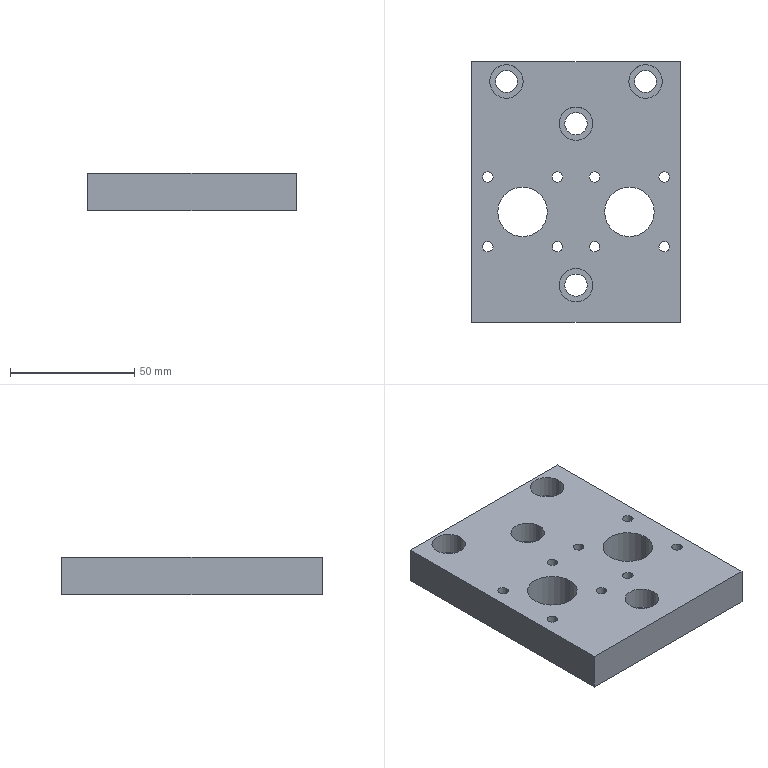Part | STEP file | Printing cylinder fixing plate | 1 solid | 46 faces | box 84 x 105 x 15 mm | volume 114533 mm3 | cylinder 36 | plane 10 | commonest cylinder face diameters 4.2 x16 9 x8 13.5 x8 20 x4
STEP:
#1=CARTESIAN_POINT('',(-9.6,6.,-7.5));
#2=VERTEX_POINT('',#1);
#3=CARTESIAN_POINT('',(-5.4,6.,-7.5));
#4=VERTEX_POINT('',#3);
#5=CARTESIAN_POINT('',(-7.5,6.,-7.5));
#6=DIRECTION('',(0.,0.,1.));
#7=DIRECTION('',(1.,0.,0.));
#8=AXIS2_PLACEMENT_3D('',#5,#6,#7);
#9=CIRCLE('',#8,2.1);
#10=EDGE_CURVE('',#2,#4,#9,.T.);
#11=ORIENTED_EDGE('',*,*,#10,.F.);
#12=CARTESIAN_POINT('',(-9.6,6.,7.5));
#13=VERTEX_POINT('',#12);
#14=CARTESIAN_POINT('',(-9.6,6.,7.5));
#15=DIRECTION('',(0.,0.,1.));
#16=VECTOR('',#15,1000.);
#17=LINE('',#14,#16);
#18=EDGE_CURVE('',#2,#13,#17,.T.);
#19=ORIENTED_EDGE('',*,*,#18,.T.);
#20=CARTESIAN_POINT('',(-5.4,6.,7.5));
#21=VERTEX_POINT('',#20);
#22=CARTESIAN_POINT('',(-7.5,6.,7.5));
#23=DIRECTION('',(0.,0.,1.));
#24=DIRECTION('',(1.,0.,0.));
#25=AXIS2_PLACEMENT_3D('',#22,#23,#24);
#26=CIRCLE('',#25,2.1);
#27=EDGE_CURVE('',#13,#21,#26,.T.);
#28=ORIENTED_EDGE('',*,*,#27,.T.);
#29=CARTESIAN_POINT('',(-5.4,6.,7.5));
#30=DIRECTION('',(0.,0.,1.));
#31=VECTOR('',#30,1000.);
#32=LINE('',#29,#31);
#33=EDGE_CURVE('',#4,#21,#32,.T.);
#34=ORIENTED_EDGE('',*,*,#33,.F.);
#35=EDGE_LOOP('',(#11,#19,#28,#34));
#36=FACE_OUTER_BOUND('',#35,.T.);
#37=CARTESIAN_POINT('',(-7.5,6.,7.5));
#38=DIRECTION('',(0.,0.,1.));
#39=DIRECTION('',(1.,0.,0.));
#40=AXIS2_PLACEMENT_3D('',#37,#38,#39);
#41=CYLINDRICAL_SURFACE('',#40,2.1);
#42=ADVANCED_FACE('',(#36),#41,.F.);
#43=CARTESIAN_POINT('',(-37.6,6.,-7.5));
#44=VERTEX_POINT('',#43);
#45=CARTESIAN_POINT('',(-33.4,6.,-7.5));
#46=VERTEX_POINT('',#45);
#47=CARTESIAN_POINT('',(-35.5,6.,-7.5));
#48=DIRECTION('',(0.,0.,1.));
#49=DIRECTION('',(1.,0.,0.));
#50=AXIS2_PLACEMENT_3D('',#47,#48,#49);
#51=CIRCLE('',#50,2.1);
#52=EDGE_CURVE('',#44,#46,#51,.T.);
#53=ORIENTED_EDGE('',*,*,#52,.F.);
#54=CARTESIAN_POINT('',(-37.6,6.,7.5));
#55=VERTEX_POINT('',#54);
#56=CARTESIAN_POINT('',(-37.6,6.,7.5));
#57=DIRECTION('',(0.,0.,1.));
#58=VECTOR('',#57,1000.);
#59=LINE('',#56,#58);
#60=EDGE_CURVE('',#44,#55,#59,.T.);
#61=ORIENTED_EDGE('',*,*,#60,.T.);
#62=CARTESIAN_POINT('',(-33.4,6.,7.5));
#63=VERTEX_POINT('',#62);
#64=CARTESIAN_POINT('',(-35.5,6.,7.5));
#65=DIRECTION('',(0.,0.,1.));
#66=DIRECTION('',(1.,0.,0.));
#67=AXIS2_PLACEMENT_3D('',#64,#65,#66);
#68=CIRCLE('',#67,2.1);
#69=EDGE_CURVE('',#55,#63,#68,.T.);
#70=ORIENTED_EDGE('',*,*,#69,.T.);
#71=CARTESIAN_POINT('',(-33.4,6.,7.5));
#72=DIRECTION('',(0.,0.,1.));
#73=VECTOR('',#72,1000.);
#74=LINE('',#71,#73);
#75=EDGE_CURVE('',#46,#63,#74,.T.);
#76=ORIENTED_EDGE('',*,*,#75,.F.);
#77=EDGE_LOOP('',(#53,#61,#70,#76));
#78=FACE_OUTER_BOUND('',#77,.T.);
#79=CARTESIAN_POINT('',(-35.5,6.,7.5));
#80=DIRECTION('',(0.,0.,1.));
#81=DIRECTION('',(1.,0.,0.));
#82=AXIS2_PLACEMENT_3D('',#79,#80,#81);
#83=CYLINDRICAL_SURFACE('',#82,2.1);
#84=ADVANCED_FACE('',(#78),#83,.F.);
#85=CARTESIAN_POINT('',(-37.6,-22.,-7.5));
#86=VERTEX_POINT('',#85);
#87=CARTESIAN_POINT('',(-33.4,-22.,-7.5));
#88=VERTEX_POINT('',#87);
#89=CARTESIAN_POINT('',(-35.5,-22.,-7.5));
#90=DIRECTION('',(0.,0.,1.));
#91=DIRECTION('',(1.,0.,0.));
#92=AXIS2_PLACEMENT_3D('',#89,#90,#91);
#93=CIRCLE('',#92,2.1);
#94=EDGE_CURVE('',#86,#88,#93,.T.);
#95=ORIENTED_EDGE('',*,*,#94,.F.);
#96=CARTESIAN_POINT('',(-37.6,-22.,7.5));
#97=VERTEX_POINT('',#96);
#98=CARTESIAN_POINT('',(-37.6,-22.,7.5));
#99=DIRECTION('',(0.,0.,1.));
#100=VECTOR('',#99,1000.);
#101=LINE('',#98,#100);
#102=EDGE_CURVE('',#86,#97,#101,.T.);
#103=ORIENTED_EDGE('',*,*,#102,.T.);
#104=CARTESIAN_POINT('',(-33.4,-22.,7.5));
#105=VERTEX_POINT('',#104);
#106=CARTESIAN_POINT('',(-35.5,-22.,7.5));
#107=DIRECTION('',(0.,0.,1.));
#108=DIRECTION('',(1.,0.,0.));
#109=AXIS2_PLACEMENT_3D('',#106,#107,#108);
#110=CIRCLE('',#109,2.1);
#111=EDGE_CURVE('',#97,#105,#110,.T.);
#112=ORIENTED_EDGE('',*,*,#111,.T.);
#113=CARTESIAN_POINT('',(-33.4,-22.,7.5));
#114=DIRECTION('',(0.,0.,1.));
#115=VECTOR('',#114,1000.);
#116=LINE('',#113,#115);
#117=EDGE_CURVE('',#88,#105,#116,.T.);
#118=ORIENTED_EDGE('',*,*,#117,.F.);
#119=EDGE_LOOP('',(#95,#103,#112,#118));
#120=FACE_OUTER_BOUND('',#119,.T.);
#121=CARTESIAN_POINT('',(-35.5,-22.,7.5));
#122=DIRECTION('',(0.,0.,1.));
#123=DIRECTION('',(1.,0.,0.));
#124=AXIS2_PLACEMENT_3D('',#121,#122,#123);
#125=CYLINDRICAL_SURFACE('',#124,2.1);
#126=ADVANCED_FACE('',(#120),#125,.F.);
#127=CARTESIAN_POINT('',(-9.6,-22.,-7.5));
#128=VERTEX_POINT('',#127);
#129=CARTESIAN_POINT('',(-5.4,-22.,-7.5));
#130=VERTEX_POINT('',#129);
#131=CARTESIAN_POINT('',(-7.5,-22.,-7.5));
#132=DIRECTION('',(0.,0.,1.));
#133=DIRECTION('',(1.,0.,0.));
#134=AXIS2_PLACEMENT_3D('',#131,#132,#133);
#135=CIRCLE('',#134,2.1);
#136=EDGE_CURVE('',#128,#130,#135,.T.);
#137=ORIENTED_EDGE('',*,*,#136,.F.);
#138=CARTESIAN_POINT('',(-9.6,-22.,7.5));
#139=VERTEX_POINT('',#138);
#140=CARTESIAN_POINT('',(-9.6,-22.,7.5));
#141=DIRECTION('',(0.,0.,1.));
#142=VECTOR('',#141,1000.);
#143=LINE('',#140,#142);
#144=EDGE_CURVE('',#128,#139,#143,.T.);
#145=ORIENTED_EDGE('',*,*,#144,.T.);
#146=CARTESIAN_POINT('',(-5.4,-22.,7.5));
#147=VERTEX_POINT('',#146);
#148=CARTESIAN_POINT('',(-7.5,-22.,7.5));
#149=DIRECTION('',(0.,0.,1.));
#150=DIRECTION('',(1.,0.,0.));
#151=AXIS2_PLACEMENT_3D('',#148,#149,#150);
#152=CIRCLE('',#151,2.1);
#153=EDGE_CURVE('',#139,#147,#152,.T.);
#154=ORIENTED_EDGE('',*,*,#153,.T.);
#155=CARTESIAN_POINT('',(-5.4,-22.,7.5));
#156=DIRECTION('',(0.,0.,1.));
#157=VECTOR('',#156,1000.);
#158=LINE('',#155,#157);
#159=EDGE_CURVE('',#130,#147,#158,.T.);
#160=ORIENTED_EDGE('',*,*,#159,.F.);
#161=EDGE_LOOP('',(#137,#145,#154,#160));
#162=FACE_OUTER_BOUND('',#161,.T.);
#163=CARTESIAN_POINT('',(-7.5,-22.,7.5));
#164=DIRECTION('',(0.,0.,1.));
#165=DIRECTION('',(1.,0.,0.));
#166=AXIS2_PLACEMENT_3D('',#163,#164,#165);
#167=CYLINDRICAL_SURFACE('',#166,2.1);
#168=ADVANCED_FACE('',(#162),#167,.F.);
#169=CARTESIAN_POINT('',(5.4,-22.,-7.5));
#170=VERTEX_POINT('',#169);
#171=CARTESIAN_POINT('',(9.6,-22.,-7.5));
#172=VERTEX_POINT('',#171);
#173=CARTESIAN_POINT('',(7.5,-22.,-7.5));
#174=DIRECTION('',(0.,0.,1.));
#175=DIRECTION('',(1.,0.,0.));
#176=AXIS2_PLACEMENT_3D('',#173,#174,#175);
#177=CIRCLE('',#176,2.1);
#178=EDGE_CURVE('',#170,#172,#177,.T.);
#179=ORIENTED_EDGE('',*,*,#178,.F.);
#180=CARTESIAN_POINT('',(5.4,-22.,7.5));
#181=VERTEX_POINT('',#180);
#182=CARTESIAN_POINT('',(5.4,-22.,7.5));
#183=DIRECTION('',(0.,0.,1.));
#184=VECTOR('',#183,1000.);
#185=LINE('',#182,#184);
#186=EDGE_CURVE('',#170,#181,#185,.T.);
#187=ORIENTED_EDGE('',*,*,#186,.T.);
#188=CARTESIAN_POINT('',(9.6,-22.,7.5));
#189=VERTEX_POINT('',#188);
#190=CARTESIAN_POINT('',(7.5,-22.,7.5));
#191=DIRECTION('',(0.,0.,1.));
#192=DIRECTION('',(1.,0.,0.));
#193=AXIS2_PLACEMENT_3D('',#190,#191,#192);
#194=CIRCLE('',#193,2.1);
#195=EDGE_CURVE('',#181,#189,#194,.T.);
#196=ORIENTED_EDGE('',*,*,#195,.T.);
#197=CARTESIAN_POINT('',(9.6,-22.,7.5));
#198=DIRECTION('',(0.,0.,1.));
#199=VECTOR('',#198,1000.);
#200=LINE('',#197,#199);
#201=EDGE_CURVE('',#172,#189,#200,.T.);
#202=ORIENTED_EDGE('',*,*,#201,.F.);
#203=EDGE_LOOP('',(#179,#187,#196,#202));
#204=FACE_OUTER_BOUND('',#203,.T.);
#205=CARTESIAN_POINT('',(7.5,-22.,7.5));
#206=DIRECTION('',(0.,0.,1.));
#207=DIRECTION('',(1.,0.,0.));
#208=AXIS2_PLACEMENT_3D('',#205,#206,#207);
#209=CYLINDRICAL_SURFACE('',#208,2.1);
#210=ADVANCED_FACE('',(#204),#209,.F.);
#211=CARTESIAN_POINT('',(33.4,-22.,-7.5));
#212=VERTEX_POINT('',#211);
#213=CARTESIAN_POINT('',(37.6,-22.,-7.5));
#214=VERTEX_POINT('',#213);
#215=CARTESIAN_POINT('',(35.5,-22.,-7.5));
#216=DIRECTION('',(0.,0.,1.));
#217=DIRECTION('',(1.,0.,0.));
#218=AXIS2_PLACEMENT_3D('',#215,#216,#217);
#219=CIRCLE('',#218,2.1);
#220=EDGE_CURVE('',#212,#214,#219,.T.);
#221=ORIENTED_EDGE('',*,*,#220,.F.);
#222=CARTESIAN_POINT('',(33.4,-22.,7.5));
#223=VERTEX_POINT('',#222);
#224=CARTESIAN_POINT('',(33.4,-22.,7.5));
#225=DIRECTION('',(0.,0.,1.));
#226=VECTOR('',#225,1000.);
#227=LINE('',#224,#226);
#228=EDGE_CURVE('',#212,#223,#227,.T.);
#229=ORIENTED_EDGE('',*,*,#228,.T.);
#230=CARTESIAN_POINT('',(37.6,-22.,7.5));
#231=VERTEX_POINT('',#230);
#232=CARTESIAN_POINT('',(35.5,-22.,7.5));
#233=DIRECTION('',(0.,0.,1.));
#234=DIRECTION('',(1.,0.,0.));
#235=AXIS2_PLACEMENT_3D('',#232,#233,#234);
#236=CIRCLE('',#235,2.1);
#237=EDGE_CURVE('',#223,#231,#236,.T.);
#238=ORIENTED_EDGE('',*,*,#237,.T.);
#239=CARTESIAN_POINT('',(37.6,-22.,7.5));
#240=DIRECTION('',(0.,0.,1.));
#241=VECTOR('',#240,1000.);
#242=LINE('',#239,#241);
#243=EDGE_CURVE('',#214,#231,#242,.T.);
#244=ORIENTED_EDGE('',*,*,#243,.F.);
#245=EDGE_LOOP('',(#221,#229,#238,#244));
#246=FACE_OUTER_BOUND('',#245,.T.);
#247=CARTESIAN_POINT('',(35.5,-22.,7.5));
#248=DIRECTION('',(0.,0.,1.));
#249=DIRECTION('',(1.,0.,0.));
#250=AXIS2_PLACEMENT_3D('',#247,#248,#249);
#251=CYLINDRICAL_SURFACE('',#250,2.1);
#252=ADVANCED_FACE('',(#246),#251,.F.);
#253=CARTESIAN_POINT('',(33.4,6.,-7.5));
#254=VERTEX_POINT('',#253);
#255=CARTESIAN_POINT('',(37.6,6.,-7.5));
#256=VERTEX_POINT('',#255);
#257=CARTESIAN_POINT('',(35.5,6.,-7.5));
#258=DIRECTION('',(0.,0.,1.));
#259=DIRECTION('',(1.,0.,0.));
#260=AXIS2_PLACEMENT_3D('',#257,#258,#259);
#261=CIRCLE('',#260,2.1);
#262=EDGE_CURVE('',#254,#256,#261,.T.);
#263=ORIENTED_EDGE('',*,*,#262,.F.);
#264=CARTESIAN_POINT('',(33.4,6.,7.5));
#265=VERTEX_POINT('',#264);
#266=CARTESIAN_POINT('',(33.4,6.,7.5));
#267=DIRECTION('',(0.,0.,1.));
#268=VECTOR('',#267,1000.);
#269=LINE('',#266,#268);
#270=EDGE_CURVE('',#254,#265,#269,.T.);
#271=ORIENTED_EDGE('',*,*,#270,.T.);
#272=CARTESIAN_POINT('',(37.6,6.,7.5));
#273=VERTEX_POINT('',#272);
#274=CARTESIAN_POINT('',(35.5,6.,7.5));
#275=DIRECTION('',(0.,0.,1.));
#276=DIRECTION('',(1.,0.,0.));
#277=AXIS2_PLACEMENT_3D('',#274,#275,#276);
#278=CIRCLE('',#277,2.1);
#279=EDGE_CURVE('',#265,#273,#278,.T.);
#280=ORIENTED_EDGE('',*,*,#279,.T.);
#281=CARTESIAN_POINT('',(37.6,6.,7.5));
#282=DIRECTION('',(0.,0.,1.));
#283=VECTOR('',#282,1000.);
#284=LINE('',#281,#283);
#285=EDGE_CURVE('',#256,#273,#284,.T.);
#286=ORIENTED_EDGE('',*,*,#285,.F.);
#287=EDGE_LOOP('',(#263,#271,#280,#286));
#288=FACE_OUTER_BOUND('',#287,.T.);
#289=CARTESIAN_POINT('',(35.5,6.,7.5));
#290=DIRECTION('',(0.,0.,1.));
#291=DIRECTION('',(1.,0.,0.));
#292=AXIS2_PLACEMENT_3D('',#289,#290,#291);
#293=CYLINDRICAL_SURFACE('',#292,2.1);
#294=ADVANCED_FACE('',(#288),#293,.F.);
#295=CARTESIAN_POINT('',(5.4,6.,-7.5));
#296=VERTEX_POINT('',#295);
#297=CARTESIAN_POINT('',(9.6,6.,-7.5));
#298=VERTEX_POINT('',#297);
#299=CARTESIAN_POINT('',(7.5,6.,-7.5));
#300=DIRECTION('',(0.,0.,1.));
#301=DIRECTION('',(1.,0.,0.));
#302=AXIS2_PLACEMENT_3D('',#299,#300,#301);
#303=CIRCLE('',#302,2.1);
#304=EDGE_CURVE('',#296,#298,#303,.T.);
#305=ORIENTED_EDGE('',*,*,#304,.F.);
#306=CARTESIAN_POINT('',(5.4,6.,7.5));
#307=VERTEX_POINT('',#306);
#308=CARTESIAN_POINT('',(5.4,6.,7.5));
#309=DIRECTION('',(0.,0.,1.));
#310=VECTOR('',#309,1000.);
#311=LINE('',#308,#310);
#312=EDGE_CURVE('',#296,#307,#311,.T.);
#313=ORIENTED_EDGE('',*,*,#312,.T.);
#314=CARTESIAN_POINT('',(9.6,6.,7.5));
#315=VERTEX_POINT('',#314);
#316=CARTESIAN_POINT('',(7.5,6.,7.5));
#317=DIRECTION('',(0.,0.,1.));
#318=DIRECTION('',(1.,0.,0.));
#319=AXIS2_PLACEMENT_3D('',#316,#317,#318);
#320=CIRCLE('',#319,2.1);
#321=EDGE_CURVE('',#307,#315,#320,.T.);
#322=ORIENTED_EDGE('',*,*,#321,.T.);
#323=CARTESIAN_POINT('',(9.6,6.,7.5));
#324=DIRECTION('',(0.,0.,1.));
#325=VECTOR('',#324,1000.);
#326=LINE('',#323,#325);
#327=EDGE_CURVE('',#298,#315,#326,.T.);
#328=ORIENTED_EDGE('',*,*,#327,.F.);
#329=EDGE_LOOP('',(#305,#313,#322,#328));
#330=FACE_OUTER_BOUND('',#329,.T.);
#331=CARTESIAN_POINT('',(7.5,6.,7.5));
#332=DIRECTION('',(0.,0.,1.));
#333=DIRECTION('',(1.,0.,0.));
#334=AXIS2_PLACEMENT_3D('',#331,#332,#333);
#335=CYLINDRICAL_SURFACE('',#334,2.1);
#336=ADVANCED_FACE('',(#330),#335,.F.);
#337=CARTESIAN_POINT('',(-34.75,44.5,-1.5));
#338=VERTEX_POINT('',#337);
#339=CARTESIAN_POINT('',(-21.25,44.5,-1.5));
#340=VERTEX_POINT('',#339);
#341=CARTESIAN_POINT('',(-28.,44.5,-1.5));
#342=DIRECTION('',(0.,0.,1.));
#343=DIRECTION('',(1.,0.,0.));
#344=AXIS2_PLACEMENT_3D('',#341,#342,#343);
#345=CIRCLE('',#344,6.75);
#346=EDGE_CURVE('',#338,#340,#345,.T.);
#347=ORIENTED_EDGE('',*,*,#346,.F.);
#348=CARTESIAN_POINT('',(-34.75,44.5,7.5));
#349=VERTEX_POINT('',#348);
#350=CARTESIAN_POINT('',(-34.75,44.5,7.5));
#351=DIRECTION('',(0.,0.,1.));
#352=VECTOR('',#351,1000.);
#353=LINE('',#350,#352);
#354=EDGE_CURVE('',#338,#349,#353,.T.);
#355=ORIENTED_EDGE('',*,*,#354,.T.);
#356=CARTESIAN_POINT('',(-21.25,44.5,7.5));
#357=VERTEX_POINT('',#356);
#358=CARTESIAN_POINT('',(-28.,44.5,7.5));
#359=DIRECTION('',(0.,0.,1.));
#360=DIRECTION('',(1.,0.,0.));
#361=AXIS2_PLACEMENT_3D('',#358,#359,#360);
#362=CIRCLE('',#361,6.75);
#363=EDGE_CURVE('',#349,#357,#362,.T.);
#364=ORIENTED_EDGE('',*,*,#363,.T.);
#365=CARTESIAN_POINT('',(-21.25,44.5,7.5));
#366=DIRECTION('',(0.,0.,1.));
#367=VECTOR('',#366,1000.);
#368=LINE('',#365,#367);
#369=EDGE_CURVE('',#340,#357,#368,.T.);
#370=ORIENTED_EDGE('',*,*,#369,.F.);
#371=EDGE_LOOP('',(#347,#355,#364,#370));
#372=FACE_OUTER_BOUND('',#371,.T.);
#373=CARTESIAN_POINT('',(-28.,44.5,7.5));
#374=DIRECTION('',(0.,0.,1.));
#375=DIRECTION('',(1.,0.,0.));
#376=AXIS2_PLACEMENT_3D('',#373,#374,#375);
#377=CYLINDRICAL_SURFACE('',#376,6.75);
#378=ADVANCED_FACE('',(#372),#377,.F.);
#379=CARTESIAN_POINT('',(-32.5,44.5,-7.5));
#380=VERTEX_POINT('',#379);
#381=CARTESIAN_POINT('',(-23.5,44.5,-7.5));
#382=VERTEX_POINT('',#381);
#383=CARTESIAN_POINT('',(-28.,44.5,-7.5));
#384=DIRECTION('',(0.,0.,1.));
#385=DIRECTION('',(1.,0.,0.));
#386=AXIS2_PLACEMENT_3D('',#383,#384,#385);
#387=CIRCLE('',#386,4.5);
#388=EDGE_CURVE('',#380,#382,#387,.T.);
#389=ORIENTED_EDGE('',*,*,#388,.F.);
#390=CARTESIAN_POINT('',(-32.5,44.5,-1.5));
#391=VERTEX_POINT('',#390);
#392=CARTESIAN_POINT('',(-32.5,44.5,7.5));
#393=DIRECTION('',(0.,0.,1.));
#394=VECTOR('',#393,1000.);
#395=LINE('',#392,#394);
#396=EDGE_CURVE('',#380,#391,#395,.T.);
#397=ORIENTED_EDGE('',*,*,#396,.T.);
#398=CARTESIAN_POINT('',(-23.5,44.5,-1.5));
#399=VERTEX_POINT('',#398);
#400=CARTESIAN_POINT('',(-28.,44.5,-1.5));
#401=DIRECTION('',(0.,0.,1.));
#402=DIRECTION('',(1.,0.,0.));
#403=AXIS2_PLACEMENT_3D('',#400,#401,#402);
#404=CIRCLE('',#403,4.5);
#405=EDGE_CURVE('',#391,#399,#404,.T.);
#406=ORIENTED_EDGE('',*,*,#405,.T.);
#407=CARTESIAN_POINT('',(-23.5,44.5,7.5));
#408=DIRECTION('',(0.,0.,1.));
#409=VECTOR('',#408,1000.);
#410=LINE('',#407,#409);
#411=EDGE_CURVE('',#382,#399,#410,.T.);
#412=ORIENTED_EDGE('',*,*,#411,.F.);
#413=EDGE_LOOP('',(#389,#397,#406,#412));
#414=FACE_OUTER_BOUND('',#413,.T.);
#415=CARTESIAN_POINT('',(-28.,44.5,7.5));
#416=DIRECTION('',(0.,0.,1.));
#417=DIRECTION('',(1.,0.,0.));
#418=AXIS2_PLACEMENT_3D('',#415,#416,#417);
#419=CYLINDRICAL_SURFACE('',#418,4.5);
#420=ADVANCED_FACE('',(#414),#419,.F.);
#421=CARTESIAN_POINT('',(21.25,44.5,-1.5));
#422=VERTEX_POINT('',#421);
#423=CARTESIAN_POINT('',(34.75,44.5,-1.5));
#424=VERTEX_POINT('',#423);
#425=CARTESIAN_POINT('',(28.,44.5,-1.5));
#426=DIRECTION('',(0.,0.,1.));
#427=DIRECTION('',(1.,0.,0.));
#428=AXIS2_PLACEMENT_3D('',#425,#426,#427);
#429=CIRCLE('',#428,6.75);
#430=EDGE_CURVE('',#422,#424,#429,.T.);
#431=ORIENTED_EDGE('',*,*,#430,.F.);
#432=CARTESIAN_POINT('',(21.25,44.5,7.5));
#433=VERTEX_POINT('',#432);
#434=CARTESIAN_POINT('',(21.25,44.5,7.5));
#435=DIRECTION('',(0.,0.,1.));
#436=VECTOR('',#435,1000.);
#437=LINE('',#434,#436);
#438=EDGE_CURVE('',#422,#433,#437,.T.);
#439=ORIENTED_EDGE('',*,*,#438,.T.);
#440=CARTESIAN_POINT('',(34.75,44.5,7.5));
#441=VERTEX_POINT('',#440);
#442=CARTESIAN_POINT('',(28.,44.5,7.5));
#443=DIRECTION('',(0.,0.,1.));
#444=DIRECTION('',(1.,0.,0.));
#445=AXIS2_PLACEMENT_3D('',#442,#443,#444);
#446=CIRCLE('',#445,6.75);
#447=EDGE_CURVE('',#433,#441,#446,.T.);
#448=ORIENTED_EDGE('',*,*,#447,.T.);
#449=CARTESIAN_POINT('',(34.75,44.5,7.5));
#450=DIRECTION('',(0.,0.,1.));
#451=VECTOR('',#450,1000.);
#452=LINE('',#449,#451);
#453=EDGE_CURVE('',#424,#441,#452,.T.);
#454=ORIENTED_EDGE('',*,*,#453,.F.);
#455=EDGE_LOOP('',(#431,#439,#448,#454));
#456=FACE_OUTER_BOUND('',#455,.T.);
#457=CARTESIAN_POINT('',(28.,44.5,7.5));
#458=DIRECTION('',(0.,0.,1.));
#459=DIRECTION('',(1.,0.,0.));
#460=AXIS2_PLACEMENT_3D('',#457,#458,#459);
#461=CYLINDRICAL_SURFACE('',#460,6.75);
#462=ADVANCED_FACE('',(#456),#461,.F.);
#463=CARTESIAN_POINT('',(23.5,44.5,-7.5));
#464=VERTEX_POINT('',#463);
#465=CARTESIAN_POINT('',(32.5,44.5,-7.5));
#466=VERTEX_POINT('',#465);
#467=CARTESIAN_POINT('',(28.,44.5,-7.5));
#468=DIRECTION('',(0.,0.,1.));
#469=DIRECTION('',(1.,0.,0.));
#470=AXIS2_PLACEMENT_3D('',#467,#468,#469);
#471=CIRCLE('',#470,4.5);
#472=EDGE_CURVE('',#464,#466,#471,.T.);
#473=ORIENTED_EDGE('',*,*,#472,.F.);
#474=CARTESIAN_POINT('',(23.5,44.5,-1.5));
#475=VERTEX_POINT('',#474);
#476=CARTESIAN_POINT('',(23.5,44.5,7.5));
#477=DIRECTION('',(0.,0.,1.));
#478=VECTOR('',#477,1000.);
#479=LINE('',#476,#478);
#480=EDGE_CURVE('',#464,#475,#479,.T.);
#481=ORIENTED_EDGE('',*,*,#480,.T.);
#482=CARTESIAN_POINT('',(32.5,44.5,-1.5));
#483=VERTEX_POINT('',#482);
#484=CARTESIAN_POINT('',(28.,44.5,-1.5));
#485=DIRECTION('',(0.,0.,1.));
#486=DIRECTION('',(1.,0.,0.));
#487=AXIS2_PLACEMENT_3D('',#484,#485,#486);
#488=CIRCLE('',#487,4.5);
#489=EDGE_CURVE('',#475,#483,#488,.T.);
#490=ORIENTED_EDGE('',*,*,#489,.T.);
#491=CARTESIAN_POINT('',(32.5,44.5,7.5));
#492=DIRECTION('',(0.,0.,1.));
#493=VECTOR('',#492,1000.);
#494=LINE('',#491,#493);
#495=EDGE_CURVE('',#466,#483,#494,.T.);
#496=ORIENTED_EDGE('',*,*,#495,.F.);
#497=EDGE_LOOP('',(#473,#481,#490,#496));
#498=FACE_OUTER_BOUND('',#497,.T.);
#499=CARTESIAN_POINT('',(28.,44.5,7.5));
#500=DIRECTION('',(0.,0.,1.));
#501=DIRECTION('',(1.,0.,0.));
#502=AXIS2_PLACEMENT_3D('',#499,#500,#501);
#503=CYLINDRICAL_SURFACE('',#502,4.5);
#504=ADVANCED_FACE('',(#498),#503,.F.);
#505=CARTESIAN_POINT('',(-6.75,27.5,-1.5));
#506=VERTEX_POINT('',#505);
#507=CARTESIAN_POINT('',(6.75,27.5,-1.5));
#508=VERTEX_POINT('',#507);
#509=CARTESIAN_POINT('',(0.,27.5,-1.5));
#510=DIRECTION('',(0.,0.,1.));
#511=DIRECTION('',(1.,0.,0.));
#512=AXIS2_PLACEMENT_3D('',#509,#510,#511);
#513=CIRCLE('',#512,6.75);
#514=EDGE_CURVE('',#506,#508,#513,.T.);
#515=ORIENTED_EDGE('',*,*,#514,.F.);
#516=CARTESIAN_POINT('',(-6.75,27.5,7.5));
#517=VERTEX_POINT('',#516);
#518=CARTESIAN_POINT('',(-6.75,27.5,7.5));
#519=DIRECTION('',(0.,0.,1.));
#520=VECTOR('',#519,1000.);
#521=LINE('',#518,#520);
#522=EDGE_CURVE('',#506,#517,#521,.T.);
#523=ORIENTED_EDGE('',*,*,#522,.T.);
#524=CARTESIAN_POINT('',(6.75,27.5,7.5));
#525=VERTEX_POINT('',#524);
#526=CARTESIAN_POINT('',(0.,27.5,7.5));
#527=DIRECTION('',(0.,0.,1.));
#528=DIRECTION('',(1.,0.,0.));
#529=AXIS2_PLACEMENT_3D('',#526,#527,#528);
#530=CIRCLE('',#529,6.75);
#531=EDGE_CURVE('',#517,#525,#530,.T.);
#532=ORIENTED_EDGE('',*,*,#531,.T.);
#533=CARTESIAN_POINT('',(6.75,27.5,7.5));
#534=DIRECTION('',(0.,0.,1.));
#535=VECTOR('',#534,1000.);
#536=LINE('',#533,#535);
#537=EDGE_CURVE('',#508,#525,#536,.T.);
#538=ORIENTED_EDGE('',*,*,#537,.F.);
#539=EDGE_LOOP('',(#515,#523,#532,#538));
#540=FACE_OUTER_BOUND('',#539,.T.);
#541=CARTESIAN_POINT('',(0.,27.5,7.5));
#542=DIRECTION('',(0.,0.,1.));
#543=DIRECTION('',(1.,0.,0.));
#544=AXIS2_PLACEMENT_3D('',#541,#542,#543);
#545=CYLINDRICAL_SURFACE('',#544,6.75);
#546=ADVANCED_FACE('',(#540),#545,.F.);
#547=CARTESIAN_POINT('',(-4.5,27.5,-7.5));
#548=VERTEX_POINT('',#547);
#549=CARTESIAN_POINT('',(4.5,27.5,-7.5));
#550=VERTEX_POINT('',#549);
#551=CARTESIAN_POINT('',(0.,27.5,-7.5));
#552=DIRECTION('',(0.,0.,1.));
#553=DIRECTION('',(1.,0.,0.));
#554=AXIS2_PLACEMENT_3D('',#551,#552,#553);
#555=CIRCLE('',#554,4.5);
#556=EDGE_CURVE('',#548,#550,#555,.T.);
#557=ORIENTED_EDGE('',*,*,#556,.F.);
#558=CARTESIAN_POINT('',(-4.5,27.5,-1.5));
#559=VERTEX_POINT('',#558);
#560=CARTESIAN_POINT('',(-4.5,27.5,7.5));
#561=DIRECTION('',(0.,0.,1.));
#562=VECTOR('',#561,1000.);
#563=LINE('',#560,#562);
#564=EDGE_CURVE('',#548,#559,#563,.T.);
#565=ORIENTED_EDGE('',*,*,#564,.T.);
#566=CARTESIAN_POINT('',(4.5,27.5,-1.5));
#567=VERTEX_POINT('',#566);
#568=CARTESIAN_POINT('',(0.,27.5,-1.5));
#569=DIRECTION('',(0.,0.,1.));
#570=DIRECTION('',(1.,0.,0.));
#571=AXIS2_PLACEMENT_3D('',#568,#569,#570);
#572=CIRCLE('',#571,4.5);
#573=EDGE_CURVE('',#559,#567,#572,.T.);
#574=ORIENTED_EDGE('',*,*,#573,.T.);
#575=CARTESIAN_POINT('',(4.5,27.5,7.5));
#576=DIRECTION('',(0.,0.,1.));
#577=VECTOR('',#576,1000.);
#578=LINE('',#575,#577);
#579=EDGE_CURVE('',#550,#567,#578,.T.);
#580=ORIENTED_EDGE('',*,*,#579,.F.);
#581=EDGE_LOOP('',(#557,#565,#574,#580));
#582=FACE_OUTER_BOUND('',#581,.T.);
#583=CARTESIAN_POINT('',(0.,27.5,7.5));
#584=DIRECTION('',(0.,0.,1.));
#585=DIRECTION('',(1.,0.,0.));
#586=AXIS2_PLACEMENT_3D('',#583,#584,#585);
#587=CYLINDRICAL_SURFACE('',#586,4.5);
#588=ADVANCED_FACE('',(#582),#587,.F.);
#589=CARTESIAN_POINT('',(-6.75,-37.5,-1.5));
#590=VERTEX_POINT('',#589);
#591=CARTESIAN_POINT('',(6.75,-37.5,-1.5));
#592=VERTEX_POINT('',#591);
#593=CARTESIAN_POINT('',(0.,-37.5,-1.5));
#594=DIRECTION('',(0.,0.,1.));
#595=DIRECTION('',(1.,0.,0.));
#596=AXIS2_PLACEMENT_3D('',#593,#594,#595);
#597=CIRCLE('',#596,6.75);
#598=EDGE_CURVE('',#590,#592,#597,.T.);
#599=ORIENTED_EDGE('',*,*,#598,.F.);
#600=CARTESIAN_POINT('',(-6.75,-37.5,7.5));
#601=VERTEX_POINT('',#600);
#602=CARTESIAN_POINT('',(-6.75,-37.5,7.5));
#603=DIRECTION('',(0.,0.,1.));
#604=VECTOR('',#603,1000.);
#605=LINE('',#602,#604);
#606=EDGE_CURVE('',#590,#601,#605,.T.);
#607=ORIENTED_EDGE('',*,*,#606,.T.);
#608=CARTESIAN_POINT('',(6.75,-37.5,7.5));
#609=VERTEX_POINT('',#608);
#610=CARTESIAN_POINT('',(0.,-37.5,7.5));
#611=DIRECTION('',(0.,0.,1.));
#612=DIRECTION('',(1.,0.,0.));
#613=AXIS2_PLACEMENT_3D('',#610,#611,#612);
#614=CIRCLE('',#613,6.75);
#615=EDGE_CURVE('',#601,#609,#614,.T.);
#616=ORIENTED_EDGE('',*,*,#615,.T.);
#617=CARTESIAN_POINT('',(6.75,-37.5,7.5));
#618=DIRECTION('',(0.,0.,1.));
#619=VECTOR('',#618,1000.);
#620=LINE('',#617,#619);
#621=EDGE_CURVE('',#592,#609,#620,.T.);
#622=ORIENTED_EDGE('',*,*,#621,.F.);
#623=EDGE_LOOP('',(#599,#607,#616,#622));
#624=FACE_OUTER_BOUND('',#623,.T.);
#625=CARTESIAN_POINT('',(0.,-37.5,7.5));
#626=DIRECTION('',(0.,0.,1.));
#627=DIRECTION('',(1.,0.,0.));
#628=AXIS2_PLACEMENT_3D('',#625,#626,#627);
#629=CYLINDRICAL_SURFACE('',#628,6.75);
#630=ADVANCED_FACE('',(#624),#629,.F.);
#631=CARTESIAN_POINT('',(-4.5,-37.5,-7.5));
#632=VERTEX_POINT('',#631);
#633=CARTESIAN_POINT('',(4.5,-37.5,-7.5));
#634=VERTEX_POINT('',#633);
#635=CARTESIAN_POINT('',(0.,-37.5,-7.5));
#636=DIRECTION('',(0.,0.,1.));
#637=DIRECTION('',(1.,0.,0.));
#638=AXIS2_PLACEMENT_3D('',#635,#636,#637);
#639=CIRCLE('',#638,4.5);
#640=EDGE_CURVE('',#632,#634,#639,.T.);
#641=ORIENTED_EDGE('',*,*,#640,.F.);
#642=CARTESIAN_POINT('',(-4.5,-37.5,-1.5));
#643=VERTEX_POINT('',#642);
#644=CARTESIAN_POINT('',(-4.5,-37.5,7.5));
#645=DIRECTION('',(0.,0.,1.));
#646=VECTOR('',#645,1000.);
#647=LINE('',#644,#646);
#648=EDGE_CURVE('',#632,#643,#647,.T.);
#649=ORIENTED_EDGE('',*,*,#648,.T.);
#650=CARTESIAN_POINT('',(4.5,-37.5,-1.5));
#651=VERTEX_POINT('',#650);
#652=CARTESIAN_POINT('',(0.,-37.5,-1.5));
#653=DIRECTION('',(0.,0.,1.));
#654=DIRECTION('',(1.,0.,0.));
#655=AXIS2_PLACEMENT_3D('',#652,#653,#654);
#656=CIRCLE('',#655,4.5);
#657=EDGE_CURVE('',#643,#651,#656,.T.);
#658=ORIENTED_EDGE('',*,*,#657,.T.);
#659=CARTESIAN_POINT('',(4.5,-37.5,7.5));
#660=DIRECTION('',(0.,0.,1.));
#661=VECTOR('',#660,1000.);
#662=LINE('',#659,#661);
#663=EDGE_CURVE('',#634,#651,#662,.T.);
#664=ORIENTED_EDGE('',*,*,#663,.F.);
#665=EDGE_LOOP('',(#641,#649,#658,#664));
#666=FACE_OUTER_BOUND('',#665,.T.);
#667=CARTESIAN_POINT('',(0.,-37.5,7.5));
#668=DIRECTION('',(0.,0.,1.));
#669=DIRECTION('',(1.,0.,0.));
#670=AXIS2_PLACEMENT_3D('',#667,#668,#669);
#671=CYLINDRICAL_SURFACE('',#670,4.5);
#672=ADVANCED_FACE('',(#666),#671,.F.);
#673=CARTESIAN_POINT('',(-31.5,-8.,-7.5));
#674=VERTEX_POINT('',#673);
#675=CARTESIAN_POINT('',(-11.5,-8.,-7.5));
#676=VERTEX_POINT('',#675);
#677=CARTESIAN_POINT('',(-21.5,-8.,-7.5));
#678=DIRECTION('',(0.,0.,1.));
#679=DIRECTION('',(1.,0.,0.));
#680=AXIS2_PLACEMENT_3D('',#677,#678,#679);
#681=CIRCLE('',#680,10.);
#682=EDGE_CURVE('',#674,#676,#681,.T.);
#683=ORIENTED_EDGE('',*,*,#682,.F.);
#684=CARTESIAN_POINT('',(-31.5,-8.,7.5));
#685=VERTEX_POINT('',#684);
#686=CARTESIAN_POINT('',(-31.5,-8.,-7.5));
#687=DIRECTION('',(0.,0.,1.));
#688=VECTOR('',#687,1000.);
#689=LINE('',#686,#688);
#690=EDGE_CURVE('',#674,#685,#689,.T.);
#691=ORIENTED_EDGE('',*,*,#690,.T.);
#692=CARTESIAN_POINT('',(-11.5,-8.,7.5));
#693=VERTEX_POINT('',#692);
#694=CARTESIAN_POINT('',(-21.5,-8.,7.5));
#695=DIRECTION('',(0.,0.,1.));
#696=DIRECTION('',(1.,0.,0.));
#697=AXIS2_PLACEMENT_3D('',#694,#695,#696);
#698=CIRCLE('',#697,10.);
#699=EDGE_CURVE('',#685,#693,#698,.T.);
#700=ORIENTED_EDGE('',*,*,#699,.T.);
#701=CARTESIAN_POINT('',(-11.5,-8.,-7.5));
#702=DIRECTION('',(0.,0.,1.));
#703=VECTOR('',#702,1000.);
#704=LINE('',#701,#703);
#705=EDGE_CURVE('',#676,#693,#704,.T.);
#706=ORIENTED_EDGE('',*,*,#705,.F.);
#707=EDGE_LOOP('',(#683,#691,#700,#706));
#708=FACE_OUTER_BOUND('',#707,.T.);
#709=CARTESIAN_POINT('',(-21.5,-8.,-7.5));
#710=DIRECTION('',(0.,0.,1.));
#711=DIRECTION('',(1.,0.,0.));
#712=AXIS2_PLACEMENT_3D('',#709,#710,#711);
#713=CYLINDRICAL_SURFACE('',#712,10.);
#714=ADVANCED_FACE('',(#708),#713,.F.);
#715=CARTESIAN_POINT('',(11.5,-8.,-7.5));
#716=VERTEX_POINT('',#715);
#717=CARTESIAN_POINT('',(31.5,-8.,-7.5));
#718=VERTEX_POINT('',#717);
#719=CARTESIAN_POINT('',(21.5,-8.,-7.5));
#720=DIRECTION('',(0.,0.,1.));
#721=DIRECTION('',(1.,0.,0.));
#722=AXIS2_PLACEMENT_3D('',#719,#720,#721);
#723=CIRCLE('',#722,10.);
#724=EDGE_CURVE('',#716,#718,#723,.T.);
#725=ORIENTED_EDGE('',*,*,#724,.F.);
#726=CARTESIAN_POINT('',(11.5,-8.,7.5));
#727=VERTEX_POINT('',#726);
#728=CARTESIAN_POINT('',(11.5,-8.,-7.5));
#729=DIRECTION('',(0.,0.,1.));
#730=VECTOR('',#729,1000.);
#731=LINE('',#728,#730);
#732=EDGE_CURVE('',#716,#727,#731,.T.);
#733=ORIENTED_EDGE('',*,*,#732,.T.);
#734=CARTESIAN_POINT('',(31.5,-8.,7.5));
#735=VERTEX_POINT('',#734);
#736=CARTESIAN_POINT('',(21.5,-8.,7.5));
#737=DIRECTION('',(0.,0.,1.));
#738=DIRECTION('',(1.,0.,0.));
#739=AXIS2_PLACEMENT_3D('',#736,#737,#738);
#740=CIRCLE('',#739,10.);
#741=EDGE_CURVE('',#727,#735,#740,.T.);
#742=ORIENTED_EDGE('',*,*,#741,.T.);
#743=CARTESIAN_POINT('',(31.5,-8.,-7.5));
#744=DIRECTION('',(0.,0.,1.));
#745=VECTOR('',#744,1000.);
#746=LINE('',#743,#745);
#747=EDGE_CURVE('',#718,#735,#746,.T.);
#748=ORIENTED_EDGE('',*,*,#747,.F.);
#749=EDGE_LOOP('',(#725,#733,#742,#748));
#750=FACE_OUTER_BOUND('',#749,.T.);
#751=CARTESIAN_POINT('',(21.5,-8.,-7.5));
#752=DIRECTION('',(0.,0.,1.));
#753=DIRECTION('',(1.,0.,0.));
#754=AXIS2_PLACEMENT_3D('',#751,#752,#753);
#755=CYLINDRICAL_SURFACE('',#754,10.);
#756=ADVANCED_FACE('',(#750),#755,.F.);
#757=CARTESIAN_POINT('',(42.,-52.5,-7.5));
#758=VERTEX_POINT('',#757);
#759=CARTESIAN_POINT('',(42.,52.5,-7.5));
#760=VERTEX_POINT('',#759);
#761=CARTESIAN_POINT('',(42.,52.5,-7.5));
#762=DIRECTION('',(0.,1.,0.));
#763=VECTOR('',#762,1000.);
#764=LINE('',#761,#763);
#765=EDGE_CURVE('',#758,#760,#764,.T.);
#766=ORIENTED_EDGE('',*,*,#765,.T.);
#767=CARTESIAN_POINT('',(42.,52.5,7.5));
#768=VERTEX_POINT('',#767);
#769=CARTESIAN_POINT('',(42.,52.5,7.5));
#770=DIRECTION('',(0.,0.,-1.));
#771=VECTOR('',#770,1000.);
#772=LINE('',#769,#771);
#773=EDGE_CURVE('',#768,#760,#772,.T.);
#774=ORIENTED_EDGE('',*,*,#773,.F.);
#775=CARTESIAN_POINT('',(42.,-52.5,7.5));
#776=VERTEX_POINT('',#775);
#777=CARTESIAN_POINT('',(42.,52.5,7.5));
#778=DIRECTION('',(0.,1.,0.));
#779=VECTOR('',#778,1000.);
#780=LINE('',#777,#779);
#781=EDGE_CURVE('',#776,#768,#780,.T.);
#782=ORIENTED_EDGE('',*,*,#781,.F.);
#783=CARTESIAN_POINT('',(42.,-52.5,7.5));
#784=DIRECTION('',(0.,0.,-1.));
#785=VECTOR('',#784,1000.);
#786=LINE('',#783,#785);
#787=EDGE_CURVE('',#776,#758,#786,.T.);
#788=ORIENTED_EDGE('',*,*,#787,.T.);
#789=EDGE_LOOP('',(#766,#774,#782,#788));
#790=FACE_OUTER_BOUND('',#789,.T.);
#791=CARTESIAN_POINT('',(42.,52.5,7.5));
#792=DIRECTION('',(-1.,0.,0.));
#793=DIRECTION('',(0.,-1.,0.));
#794=AXIS2_PLACEMENT_3D('',#791,#792,#793);
#795=PLANE('',#794);
#796=ADVANCED_FACE('',(#790),#795,.F.);
#797=CARTESIAN_POINT('',(-42.,52.5,-7.5));
#798=VERTEX_POINT('',#797);
#799=CARTESIAN_POINT('',(-42.,52.5,-7.5));
#800=DIRECTION('',(-1.,0.,0.));
#801=VECTOR('',#800,1000.);
#802=LINE('',#799,#801);
#803=EDGE_CURVE('',#760,#798,#802,.T.);
#804=ORIENTED_EDGE('',*,*,#803,.T.);
#805=CARTESIAN_POINT('',(-42.,52.5,7.5));
#806=VERTEX_POINT('',#805);
#807=CARTESIAN_POINT('',(-42.,52.5,7.5));
#808=DIRECTION('',(0.,0.,-1.));
#809=VECTOR('',#808,1000.);
#810=LINE('',#807,#809);
#811=EDGE_CURVE('',#806,#798,#810,.T.);
#812=ORIENTED_EDGE('',*,*,#811,.F.);
#813=CARTESIAN_POINT('',(-42.,52.5,7.5));
#814=DIRECTION('',(-1.,0.,0.));
#815=VECTOR('',#814,1000.);
#816=LINE('',#813,#815);
#817=EDGE_CURVE('',#768,#806,#816,.T.);
#818=ORIENTED_EDGE('',*,*,#817,.F.);
#819=ORIENTED_EDGE('',*,*,#773,.T.);
#820=EDGE_LOOP('',(#804,#812,#818,#819));
#821=FACE_OUTER_BOUND('',#820,.T.);
#822=CARTESIAN_POINT('',(-42.,52.5,7.5));
#823=DIRECTION('',(0.,-1.,0.));
#824=DIRECTION('',(0.,0.,-1.));
#825=AXIS2_PLACEMENT_3D('',#822,#823,#824);
#826=PLANE('',#825);
#827=ADVANCED_FACE('',(#821),#826,.F.);
#828=CARTESIAN_POINT('',(-42.,-52.5,-7.5));
#829=VERTEX_POINT('',#828);
#830=CARTESIAN_POINT('',(-42.,52.5,-7.5));
#831=DIRECTION('',(0.,-1.,0.));
#832=VECTOR('',#831,1000.);
#833=LINE('',#830,#832);
#834=EDGE_CURVE('',#798,#829,#833,.T.);
#835=ORIENTED_EDGE('',*,*,#834,.T.);
#836=CARTESIAN_POINT('',(-42.,-52.5,7.5));
#837=VERTEX_POINT('',#836);
#838=CARTESIAN_POINT('',(-42.,-52.5,7.5));
#839=DIRECTION('',(0.,0.,-1.));
#840=VECTOR('',#839,1000.);
#841=LINE('',#838,#840);
#842=EDGE_CURVE('',#837,#829,#841,.T.);
#843=ORIENTED_EDGE('',*,*,#842,.F.);
#844=CARTESIAN_POINT('',(-42.,52.5,7.5));
#845=DIRECTION('',(0.,-1.,0.));
#846=VECTOR('',#845,1000.);
#847=LINE('',#844,#846);
#848=EDGE_CURVE('',#806,#837,#847,.T.);
#849=ORIENTED_EDGE('',*,*,#848,.F.);
#850=ORIENTED_EDGE('',*,*,#811,.T.);
#851=EDGE_LOOP('',(#835,#843,#849,#850));
#852=FACE_OUTER_BOUND('',#851,.T.);
#853=CARTESIAN_POINT('',(-42.,52.5,7.5));
#854=DIRECTION('',(1.,0.,0.));
#855=DIRECTION('',(0.,1.,0.));
#856=AXIS2_PLACEMENT_3D('',#853,#854,#855);
#857=PLANE('',#856);
#858=ADVANCED_FACE('',(#852),#857,.F.);
#859=CARTESIAN_POINT('',(-42.,-52.5,-7.5));
#860=DIRECTION('',(1.,0.,0.));
#861=VECTOR('',#860,1000.);
#862=LINE('',#859,#861);
#863=EDGE_CURVE('',#829,#758,#862,.T.);
#864=ORIENTED_EDGE('',*,*,#863,.T.);
#865=ORIENTED_EDGE('',*,*,#787,.F.);
#866=CARTESIAN_POINT('',(-42.,-52.5,7.5));
#867=DIRECTION('',(1.,0.,0.));
#868=VECTOR('',#867,1000.);
#869=LINE('',#866,#868);
#870=EDGE_CURVE('',#837,#776,#869,.T.);
#871=ORIENTED_EDGE('',*,*,#870,.F.);
#872=ORIENTED_EDGE('',*,*,#842,.T.);
#873=EDGE_LOOP('',(#864,#865,#871,#872));
#874=FACE_OUTER_BOUND('',#873,.T.);
#875=CARTESIAN_POINT('',(-42.,-52.5,7.5));
#876=DIRECTION('',(0.,1.,0.));
#877=DIRECTION('',(0.,0.,1.));
#878=AXIS2_PLACEMENT_3D('',#875,#876,#877);
#879=PLANE('',#878);
#880=ADVANCED_FACE('',(#874),#879,.F.);
#881=CARTESIAN_POINT('',(-7.5,6.,7.5));
#882=DIRECTION('',(0.,0.,1.));
#883=DIRECTION('',(1.,0.,0.));
#884=AXIS2_PLACEMENT_3D('',#881,#882,#883);
#885=CIRCLE('',#884,2.1);
#886=EDGE_CURVE('',#21,#13,#885,.T.);
#887=ORIENTED_EDGE('',*,*,#886,.F.);
#888=ORIENTED_EDGE('',*,*,#27,.F.);
#889=EDGE_LOOP('',(#887,#888));
#890=FACE_BOUND('',#889,.T.);
#891=CARTESIAN_POINT('',(-35.5,6.,7.5));
#892=DIRECTION('',(0.,0.,1.));
#893=DIRECTION('',(1.,0.,0.));
#894=AXIS2_PLACEMENT_3D('',#891,#892,#893);
#895=CIRCLE('',#894,2.1);
#896=EDGE_CURVE('',#63,#55,#895,.T.);
#897=ORIENTED_EDGE('',*,*,#896,.F.);
#898=ORIENTED_EDGE('',*,*,#69,.F.);
#899=EDGE_LOOP('',(#897,#898));
#900=FACE_BOUND('',#899,.T.);
#901=CARTESIAN_POINT('',(-35.5,-22.,7.5));
#902=DIRECTION('',(0.,0.,1.));
#903=DIRECTION('',(1.,0.,0.));
#904=AXIS2_PLACEMENT_3D('',#901,#902,#903);
#905=CIRCLE('',#904,2.1);
#906=EDGE_CURVE('',#105,#97,#905,.T.);
#907=ORIENTED_EDGE('',*,*,#906,.F.);
#908=ORIENTED_EDGE('',*,*,#111,.F.);
#909=EDGE_LOOP('',(#907,#908));
#910=FACE_BOUND('',#909,.T.);
#911=CARTESIAN_POINT('',(-7.5,-22.,7.5));
#912=DIRECTION('',(0.,0.,1.));
#913=DIRECTION('',(1.,0.,0.));
#914=AXIS2_PLACEMENT_3D('',#911,#912,#913);
#915=CIRCLE('',#914,2.1);
#916=EDGE_CURVE('',#147,#139,#915,.T.);
#917=ORIENTED_EDGE('',*,*,#916,.F.);
#918=ORIENTED_EDGE('',*,*,#153,.F.);
#919=EDGE_LOOP('',(#917,#918));
#920=FACE_BOUND('',#919,.T.);
#921=CARTESIAN_POINT('',(7.5,-22.,7.5));
#922=DIRECTION('',(0.,0.,1.));
#923=DIRECTION('',(1.,0.,0.));
#924=AXIS2_PLACEMENT_3D('',#921,#922,#923);
#925=CIRCLE('',#924,2.1);
#926=EDGE_CURVE('',#189,#181,#925,.T.);
#927=ORIENTED_EDGE('',*,*,#926,.F.);
#928=ORIENTED_EDGE('',*,*,#195,.F.);
#929=EDGE_LOOP('',(#927,#928));
#930=FACE_BOUND('',#929,.T.);
#931=CARTESIAN_POINT('',(35.5,-22.,7.5));
#932=DIRECTION('',(0.,0.,1.));
#933=DIRECTION('',(1.,0.,0.));
#934=AXIS2_PLACEMENT_3D('',#931,#932,#933);
#935=CIRCLE('',#934,2.1);
#936=EDGE_CURVE('',#231,#223,#935,.T.);
#937=ORIENTED_EDGE('',*,*,#936,.F.);
#938=ORIENTED_EDGE('',*,*,#237,.F.);
#939=EDGE_LOOP('',(#937,#938));
#940=FACE_BOUND('',#939,.T.);
#941=CARTESIAN_POINT('',(35.5,6.,7.5));
#942=DIRECTION('',(0.,0.,1.));
#943=DIRECTION('',(1.,0.,0.));
#944=AXIS2_PLACEMENT_3D('',#941,#942,#943);
#945=CIRCLE('',#944,2.1);
#946=EDGE_CURVE('',#273,#265,#945,.T.);
#947=ORIENTED_EDGE('',*,*,#946,.F.);
#948=ORIENTED_EDGE('',*,*,#279,.F.);
#949=EDGE_LOOP('',(#947,#948));
#950=FACE_BOUND('',#949,.T.);
#951=CARTESIAN_POINT('',(7.5,6.,7.5));
#952=DIRECTION('',(0.,0.,1.));
#953=DIRECTION('',(1.,0.,0.));
#954=AXIS2_PLACEMENT_3D('',#951,#952,#953);
#955=CIRCLE('',#954,2.1);
#956=EDGE_CURVE('',#315,#307,#955,.T.);
#957=ORIENTED_EDGE('',*,*,#956,.F.);
#958=ORIENTED_EDGE('',*,*,#321,.F.);
#959=EDGE_LOOP('',(#957,#958));
#960=FACE_BOUND('',#959,.T.);
#961=CARTESIAN_POINT('',(-28.,44.5,7.5));
#962=DIRECTION('',(0.,0.,1.));
#963=DIRECTION('',(1.,0.,0.));
#964=AXIS2_PLACEMENT_3D('',#961,#962,#963);
#965=CIRCLE('',#964,6.75);
#966=EDGE_CURVE('',#357,#349,#965,.T.);
#967=ORIENTED_EDGE('',*,*,#966,.F.);
#968=ORIENTED_EDGE('',*,*,#363,.F.);
#969=EDGE_LOOP('',(#967,#968));
#970=FACE_BOUND('',#969,.T.);
#971=CARTESIAN_POINT('',(28.,44.5,7.5));
#972=DIRECTION('',(0.,0.,1.));
#973=DIRECTION('',(1.,0.,0.));
#974=AXIS2_PLACEMENT_3D('',#971,#972,#973);
#975=CIRCLE('',#974,6.75);
#976=EDGE_CURVE('',#441,#433,#975,.T.);
#977=ORIENTED_EDGE('',*,*,#976,.F.);
#978=ORIENTED_EDGE('',*,*,#447,.F.);
#979=EDGE_LOOP('',(#977,#978));
#980=FACE_BOUND('',#979,.T.);
#981=CARTESIAN_POINT('',(0.,27.5,7.5));
#982=DIRECTION('',(0.,0.,1.));
#983=DIRECTION('',(1.,0.,0.));
#984=AXIS2_PLACEMENT_3D('',#981,#982,#983);
#985=CIRCLE('',#984,6.75);
#986=EDGE_CURVE('',#525,#517,#985,.T.);
#987=ORIENTED_EDGE('',*,*,#986,.F.);
#988=ORIENTED_EDGE('',*,*,#531,.F.);
#989=EDGE_LOOP('',(#987,#988));
#990=FACE_BOUND('',#989,.T.);
#991=CARTESIAN_POINT('',(0.,-37.5,7.5));
#992=DIRECTION('',(0.,0.,1.));
#993=DIRECTION('',(1.,0.,0.));
#994=AXIS2_PLACEMENT_3D('',#991,#992,#993);
#995=CIRCLE('',#994,6.75);
#996=EDGE_CURVE('',#609,#601,#995,.T.);
#997=ORIENTED_EDGE('',*,*,#996,.F.);
#998=ORIENTED_EDGE('',*,*,#615,.F.);
#999=EDGE_LOOP('',(#997,#998));
#1000=FACE_BOUND('',#999,.T.);
#1001=CARTESIAN_POINT('',(-21.5,-8.,7.5));
#1002=DIRECTION('',(0.,0.,1.));
#1003=DIRECTION('',(1.,0.,0.));
#1004=AXIS2_PLACEMENT_3D('',#1001,#1002,#1003);
#1005=CIRCLE('',#1004,10.);
#1006=EDGE_CURVE('',#693,#685,#1005,.T.);
#1007=ORIENTED_EDGE('',*,*,#1006,.F.);
#1008=ORIENTED_EDGE('',*,*,#699,.F.);
#1009=EDGE_LOOP('',(#1007,#1008));
#1010=FACE_BOUND('',#1009,.T.);
#1011=CARTESIAN_POINT('',(21.5,-8.,7.5));
#1012=DIRECTION('',(0.,0.,1.));
#1013=DIRECTION('',(1.,0.,0.));
#1014=AXIS2_PLACEMENT_3D('',#1011,#1012,#1013);
#1015=CIRCLE('',#1014,10.);
#1016=EDGE_CURVE('',#735,#727,#1015,.T.);
#1017=ORIENTED_EDGE('',*,*,#1016,.F.);
#1018=ORIENTED_EDGE('',*,*,#741,.F.);
#1019=EDGE_LOOP('',(#1017,#1018));
#1020=FACE_BOUND('',#1019,.T.);
#1021=ORIENTED_EDGE('',*,*,#781,.T.);
#1022=ORIENTED_EDGE('',*,*,#817,.T.);
#1023=ORIENTED_EDGE('',*,*,#848,.T.);
#1024=ORIENTED_EDGE('',*,*,#870,.T.);
#1025=EDGE_LOOP('',(#1021,#1022,#1023,#1024));
#1026=FACE_OUTER_BOUND('',#1025,.T.);
#1027=CARTESIAN_POINT('',(0.,0.,7.5));
#1028=DIRECTION('',(0.,0.,1.));
#1029=DIRECTION('',(1.,0.,0.));
#1030=AXIS2_PLACEMENT_3D('',#1027,#1028,#1029);
#1031=PLANE('',#1030);
#1032=ADVANCED_FACE('',(#890,#900,#910,#920,#930,#940,#950,#960,#970,#980,#990,#1000,#1010,#1020,#1026),#1031,.T.);
#1033=CARTESIAN_POINT('',(-7.5,6.,-7.5));
#1034=DIRECTION('',(0.,0.,1.));
#1035=DIRECTION('',(1.,0.,0.));
#1036=AXIS2_PLACEMENT_3D('',#1033,#1034,#1035);
#1037=CIRCLE('',#1036,2.1);
#1038=EDGE_CURVE('',#4,#2,#1037,.T.);
#1039=ORIENTED_EDGE('',*,*,#1038,.T.);
#1040=ORIENTED_EDGE('',*,*,#10,.T.);
#1041=EDGE_LOOP('',(#1039,#1040));
#1042=FACE_BOUND('',#1041,.T.);
#1043=CARTESIAN_POINT('',(-35.5,6.,-7.5));
#1044=DIRECTION('',(0.,0.,1.));
#1045=DIRECTION('',(1.,0.,0.));
#1046=AXIS2_PLACEMENT_3D('',#1043,#1044,#1045);
#1047=CIRCLE('',#1046,2.1);
#1048=EDGE_CURVE('',#46,#44,#1047,.T.);
#1049=ORIENTED_EDGE('',*,*,#1048,.T.);
#1050=ORIENTED_EDGE('',*,*,#52,.T.);
#1051=EDGE_LOOP('',(#1049,#1050));
#1052=FACE_BOUND('',#1051,.T.);
#1053=CARTESIAN_POINT('',(-35.5,-22.,-7.5));
#1054=DIRECTION('',(0.,0.,1.));
#1055=DIRECTION('',(1.,0.,0.));
#1056=AXIS2_PLACEMENT_3D('',#1053,#1054,#1055);
#1057=CIRCLE('',#1056,2.1);
#1058=EDGE_CURVE('',#88,#86,#1057,.T.);
#1059=ORIENTED_EDGE('',*,*,#1058,.T.);
#1060=ORIENTED_EDGE('',*,*,#94,.T.);
#1061=EDGE_LOOP('',(#1059,#1060));
#1062=FACE_BOUND('',#1061,.T.);
#1063=CARTESIAN_POINT('',(-7.5,-22.,-7.5));
#1064=DIRECTION('',(0.,0.,1.));
#1065=DIRECTION('',(1.,0.,0.));
#1066=AXIS2_PLACEMENT_3D('',#1063,#1064,#1065);
#1067=CIRCLE('',#1066,2.1);
#1068=EDGE_CURVE('',#130,#128,#1067,.T.);
#1069=ORIENTED_EDGE('',*,*,#1068,.T.);
#1070=ORIENTED_EDGE('',*,*,#136,.T.);
#1071=EDGE_LOOP('',(#1069,#1070));
#1072=FACE_BOUND('',#1071,.T.);
#1073=CARTESIAN_POINT('',(7.5,-22.,-7.5));
#1074=DIRECTION('',(0.,0.,1.));
#1075=DIRECTION('',(1.,0.,0.));
#1076=AXIS2_PLACEMENT_3D('',#1073,#1074,#1075);
#1077=CIRCLE('',#1076,2.1);
#1078=EDGE_CURVE('',#172,#170,#1077,.T.);
#1079=ORIENTED_EDGE('',*,*,#1078,.T.);
#1080=ORIENTED_EDGE('',*,*,#178,.T.);
#1081=EDGE_LOOP('',(#1079,#1080));
#1082=FACE_BOUND('',#1081,.T.);
#1083=CARTESIAN_POINT('',(35.5,-22.,-7.5));
#1084=DIRECTION('',(0.,0.,1.));
#1085=DIRECTION('',(1.,0.,0.));
#1086=AXIS2_PLACEMENT_3D('',#1083,#1084,#1085);
#1087=CIRCLE('',#1086,2.1);
#1088=EDGE_CURVE('',#214,#212,#1087,.T.);
#1089=ORIENTED_EDGE('',*,*,#1088,.T.);
#1090=ORIENTED_EDGE('',*,*,#220,.T.);
#1091=EDGE_LOOP('',(#1089,#1090));
#1092=FACE_BOUND('',#1091,.T.);
#1093=CARTESIAN_POINT('',(35.5,6.,-7.5));
#1094=DIRECTION('',(0.,0.,1.));
#1095=DIRECTION('',(1.,0.,0.));
#1096=AXIS2_PLACEMENT_3D('',#1093,#1094,#1095);
#1097=CIRCLE('',#1096,2.1);
#1098=EDGE_CURVE('',#256,#254,#1097,.T.);
#1099=ORIENTED_EDGE('',*,*,#1098,.T.);
#1100=ORIENTED_EDGE('',*,*,#262,.T.);
#1101=EDGE_LOOP('',(#1099,#1100));
#1102=FACE_BOUND('',#1101,.T.);
#1103=CARTESIAN_POINT('',(7.5,6.,-7.5));
#1104=DIRECTION('',(0.,0.,1.));
#1105=DIRECTION('',(1.,0.,0.));
#1106=AXIS2_PLACEMENT_3D('',#1103,#1104,#1105);
#1107=CIRCLE('',#1106,2.1);
#1108=EDGE_CURVE('',#298,#296,#1107,.T.);
#1109=ORIENTED_EDGE('',*,*,#1108,.T.);
#1110=ORIENTED_EDGE('',*,*,#304,.T.);
#1111=EDGE_LOOP('',(#1109,#1110));
#1112=FACE_BOUND('',#1111,.T.);
#1113=CARTESIAN_POINT('',(-28.,44.5,-7.5));
#1114=DIRECTION('',(0.,0.,1.));
#1115=DIRECTION('',(1.,0.,0.));
#1116=AXIS2_PLACEMENT_3D('',#1113,#1114,#1115);
#1117=CIRCLE('',#1116,4.5);
#1118=EDGE_CURVE('',#382,#380,#1117,.T.);
#1119=ORIENTED_EDGE('',*,*,#1118,.T.);
#1120=ORIENTED_EDGE('',*,*,#388,.T.);
#1121=EDGE_LOOP('',(#1119,#1120));
#1122=FACE_BOUND('',#1121,.T.);
#1123=CARTESIAN_POINT('',(28.,44.5,-7.5));
#1124=DIRECTION('',(0.,0.,1.));
#1125=DIRECTION('',(1.,0.,0.));
#1126=AXIS2_PLACEMENT_3D('',#1123,#1124,#1125);
#1127=CIRCLE('',#1126,4.5);
#1128=EDGE_CURVE('',#466,#464,#1127,.T.);
#1129=ORIENTED_EDGE('',*,*,#1128,.T.);
#1130=ORIENTED_EDGE('',*,*,#472,.T.);
#1131=EDGE_LOOP('',(#1129,#1130));
#1132=FACE_BOUND('',#1131,.T.);
#1133=CARTESIAN_POINT('',(0.,27.5,-7.5));
#1134=DIRECTION('',(0.,0.,1.));
#1135=DIRECTION('',(1.,0.,0.));
#1136=AXIS2_PLACEMENT_3D('',#1133,#1134,#1135);
#1137=CIRCLE('',#1136,4.5);
#1138=EDGE_CURVE('',#550,#548,#1137,.T.);
#1139=ORIENTED_EDGE('',*,*,#1138,.T.);
#1140=ORIENTED_EDGE('',*,*,#556,.T.);
#1141=EDGE_LOOP('',(#1139,#1140));
#1142=FACE_BOUND('',#1141,.T.);
#1143=CARTESIAN_POINT('',(0.,-37.5,-7.5));
#1144=DIRECTION('',(0.,0.,1.));
#1145=DIRECTION('',(1.,0.,0.));
#1146=AXIS2_PLACEMENT_3D('',#1143,#1144,#1145);
#1147=CIRCLE('',#1146,4.5);
#1148=EDGE_CURVE('',#634,#632,#1147,.T.);
#1149=ORIENTED_EDGE('',*,*,#1148,.T.);
#1150=ORIENTED_EDGE('',*,*,#640,.T.);
#1151=EDGE_LOOP('',(#1149,#1150));
#1152=FACE_BOUND('',#1151,.T.);
#1153=CARTESIAN_POINT('',(-21.5,-8.,-7.5));
#1154=DIRECTION('',(0.,0.,1.));
#1155=DIRECTION('',(1.,0.,0.));
#1156=AXIS2_PLACEMENT_3D('',#1153,#1154,#1155);
#1157=CIRCLE('',#1156,10.);
#1158=EDGE_CURVE('',#676,#674,#1157,.T.);
#1159=ORIENTED_EDGE('',*,*,#1158,.T.);
#1160=ORIENTED_EDGE('',*,*,#682,.T.);
#1161=EDGE_LOOP('',(#1159,#1160));
#1162=FACE_BOUND('',#1161,.T.);
#1163=CARTESIAN_POINT('',(21.5,-8.,-7.5));
#1164=DIRECTION('',(0.,0.,1.));
#1165=DIRECTION('',(1.,0.,0.));
#1166=AXIS2_PLACEMENT_3D('',#1163,#1164,#1165);
#1167=CIRCLE('',#1166,10.);
#1168=EDGE_CURVE('',#718,#716,#1167,.T.);
#1169=ORIENTED_EDGE('',*,*,#1168,.T.);
#1170=ORIENTED_EDGE('',*,*,#724,.T.);
#1171=EDGE_LOOP('',(#1169,#1170));
#1172=FACE_BOUND('',#1171,.T.);
#1173=ORIENTED_EDGE('',*,*,#765,.F.);
#1174=ORIENTED_EDGE('',*,*,#863,.F.);
#1175=ORIENTED_EDGE('',*,*,#834,.F.);
#1176=ORIENTED_EDGE('',*,*,#803,.F.);
#1177=EDGE_LOOP('',(#1173,#1174,#1175,#1176));
#1178=FACE_OUTER_BOUND('',#1177,.T.);
#1179=CARTESIAN_POINT('',(0.,0.,-7.5));
#1180=DIRECTION('',(0.,0.,1.));
#1181=DIRECTION('',(1.,0.,0.));
#1182=AXIS2_PLACEMENT_3D('',#1179,#1180,#1181);
#1183=PLANE('',#1182);
#1184=ADVANCED_FACE('',(#1042,#1052,#1062,#1072,#1082,#1092,#1102,#1112,#1122,#1132,#1142,#1152,#1162,#1172,#1178),#1183,.F.);
#1185=ORIENTED_EDGE('',*,*,#732,.F.);
#1186=ORIENTED_EDGE('',*,*,#1168,.F.);
#1187=ORIENTED_EDGE('',*,*,#747,.T.);
#1188=ORIENTED_EDGE('',*,*,#1016,.T.);
#1189=EDGE_LOOP('',(#1185,#1186,#1187,#1188));
#1190=FACE_OUTER_BOUND('',#1189,.T.);
#1191=CARTESIAN_POINT('',(21.5,-8.,-7.5));
#1192=DIRECTION('',(0.,0.,1.));
#1193=DIRECTION('',(1.,0.,0.));
#1194=AXIS2_PLACEMENT_3D('',#1191,#1192,#1193);
#1195=CYLINDRICAL_SURFACE('',#1194,10.);
#1196=ADVANCED_FACE('',(#1190),#1195,.F.);
#1197=ORIENTED_EDGE('',*,*,#690,.F.);
#1198=ORIENTED_EDGE('',*,*,#1158,.F.);
#1199=ORIENTED_EDGE('',*,*,#705,.T.);
#1200=ORIENTED_EDGE('',*,*,#1006,.T.);
#1201=EDGE_LOOP('',(#1197,#1198,#1199,#1200));
#1202=FACE_OUTER_BOUND('',#1201,.T.);
#1203=CARTESIAN_POINT('',(-21.5,-8.,-7.5));
#1204=DIRECTION('',(0.,0.,1.));
#1205=DIRECTION('',(1.,0.,0.));
#1206=AXIS2_PLACEMENT_3D('',#1203,#1204,#1205);
#1207=CYLINDRICAL_SURFACE('',#1206,10.);
#1208=ADVANCED_FACE('',(#1202),#1207,.F.);
#1209=ORIENTED_EDGE('',*,*,#648,.F.);
#1210=ORIENTED_EDGE('',*,*,#1148,.F.);
#1211=ORIENTED_EDGE('',*,*,#663,.T.);
#1212=CARTESIAN_POINT('',(0.,-37.5,-1.5));
#1213=DIRECTION('',(0.,0.,1.));
#1214=DIRECTION('',(1.,0.,0.));
#1215=AXIS2_PLACEMENT_3D('',#1212,#1213,#1214);
#1216=CIRCLE('',#1215,4.5);
#1217=EDGE_CURVE('',#651,#643,#1216,.T.);
#1218=ORIENTED_EDGE('',*,*,#1217,.T.);
#1219=EDGE_LOOP('',(#1209,#1210,#1211,#1218));
#1220=FACE_OUTER_BOUND('',#1219,.T.);
#1221=CARTESIAN_POINT('',(0.,-37.5,7.5));
#1222=DIRECTION('',(0.,0.,1.));
#1223=DIRECTION('',(1.,0.,0.));
#1224=AXIS2_PLACEMENT_3D('',#1221,#1222,#1223);
#1225=CYLINDRICAL_SURFACE('',#1224,4.5);
#1226=ADVANCED_FACE('',(#1220),#1225,.F.);
#1227=ORIENTED_EDGE('',*,*,#1217,.F.);
#1228=ORIENTED_EDGE('',*,*,#657,.F.);
#1229=EDGE_LOOP('',(#1227,#1228));
#1230=FACE_BOUND('',#1229,.T.);
#1231=CARTESIAN_POINT('',(0.,-37.5,-1.5));
#1232=DIRECTION('',(0.,0.,1.));
#1233=DIRECTION('',(1.,0.,0.));
#1234=AXIS2_PLACEMENT_3D('',#1231,#1232,#1233);
#1235=CIRCLE('',#1234,6.75);
#1236=EDGE_CURVE('',#592,#590,#1235,.T.);
#1237=ORIENTED_EDGE('',*,*,#1236,.T.);
#1238=ORIENTED_EDGE('',*,*,#598,.T.);
#1239=EDGE_LOOP('',(#1237,#1238));
#1240=FACE_OUTER_BOUND('',#1239,.T.);
#1241=CARTESIAN_POINT('',(4.5,-37.5,-1.5));
#1242=DIRECTION('',(0.,0.,-1.));
#1243=DIRECTION('',(-1.,0.,0.));
#1244=AXIS2_PLACEMENT_3D('',#1241,#1242,#1243);
#1245=PLANE('',#1244);
#1246=ADVANCED_FACE('',(#1230,#1240),#1245,.F.);
#1247=ORIENTED_EDGE('',*,*,#606,.F.);
#1248=ORIENTED_EDGE('',*,*,#1236,.F.);
#1249=ORIENTED_EDGE('',*,*,#621,.T.);
#1250=ORIENTED_EDGE('',*,*,#996,.T.);
#1251=EDGE_LOOP('',(#1247,#1248,#1249,#1250));
#1252=FACE_OUTER_BOUND('',#1251,.T.);
#1253=CARTESIAN_POINT('',(0.,-37.5,7.5));
#1254=DIRECTION('',(0.,0.,1.));
#1255=DIRECTION('',(1.,0.,0.));
#1256=AXIS2_PLACEMENT_3D('',#1253,#1254,#1255);
#1257=CYLINDRICAL_SURFACE('',#1256,6.75);
#1258=ADVANCED_FACE('',(#1252),#1257,.F.);
#1259=ORIENTED_EDGE('',*,*,#564,.F.);
#1260=ORIENTED_EDGE('',*,*,#1138,.F.);
#1261=ORIENTED_EDGE('',*,*,#579,.T.);
#1262=CARTESIAN_POINT('',(0.,27.5,-1.5));
#1263=DIRECTION('',(0.,0.,1.));
#1264=DIRECTION('',(1.,0.,0.));
#1265=AXIS2_PLACEMENT_3D('',#1262,#1263,#1264);
#1266=CIRCLE('',#1265,4.5);
#1267=EDGE_CURVE('',#567,#559,#1266,.T.);
#1268=ORIENTED_EDGE('',*,*,#1267,.T.);
#1269=EDGE_LOOP('',(#1259,#1260,#1261,#1268));
#1270=FACE_OUTER_BOUND('',#1269,.T.);
#1271=CARTESIAN_POINT('',(0.,27.5,7.5));
#1272=DIRECTION('',(0.,0.,1.));
#1273=DIRECTION('',(1.,0.,0.));
#1274=AXIS2_PLACEMENT_3D('',#1271,#1272,#1273);
#1275=CYLINDRICAL_SURFACE('',#1274,4.5);
#1276=ADVANCED_FACE('',(#1270),#1275,.F.);
#1277=ORIENTED_EDGE('',*,*,#1267,.F.);
#1278=ORIENTED_EDGE('',*,*,#573,.F.);
#1279=EDGE_LOOP('',(#1277,#1278));
#1280=FACE_BOUND('',#1279,.T.);
#1281=CARTESIAN_POINT('',(0.,27.5,-1.5));
#1282=DIRECTION('',(0.,0.,1.));
#1283=DIRECTION('',(1.,0.,0.));
#1284=AXIS2_PLACEMENT_3D('',#1281,#1282,#1283);
#1285=CIRCLE('',#1284,6.75);
#1286=EDGE_CURVE('',#508,#506,#1285,.T.);
#1287=ORIENTED_EDGE('',*,*,#1286,.T.);
#1288=ORIENTED_EDGE('',*,*,#514,.T.);
#1289=EDGE_LOOP('',(#1287,#1288));
#1290=FACE_OUTER_BOUND('',#1289,.T.);
#1291=CARTESIAN_POINT('',(4.5,27.5,-1.5));
#1292=DIRECTION('',(0.,0.,-1.));
#1293=DIRECTION('',(-1.,0.,0.));
#1294=AXIS2_PLACEMENT_3D('',#1291,#1292,#1293);
#1295=PLANE('',#1294);
#1296=ADVANCED_FACE('',(#1280,#1290),#1295,.F.);
#1297=ORIENTED_EDGE('',*,*,#522,.F.);
#1298=ORIENTED_EDGE('',*,*,#1286,.F.);
#1299=ORIENTED_EDGE('',*,*,#537,.T.);
#1300=ORIENTED_EDGE('',*,*,#986,.T.);
#1301=EDGE_LOOP('',(#1297,#1298,#1299,#1300));
#1302=FACE_OUTER_BOUND('',#1301,.T.);
#1303=CARTESIAN_POINT('',(0.,27.5,7.5));
#1304=DIRECTION('',(0.,0.,1.));
#1305=DIRECTION('',(1.,0.,0.));
#1306=AXIS2_PLACEMENT_3D('',#1303,#1304,#1305);
#1307=CYLINDRICAL_SURFACE('',#1306,6.75);
#1308=ADVANCED_FACE('',(#1302),#1307,.F.);
#1309=ORIENTED_EDGE('',*,*,#480,.F.);
#1310=ORIENTED_EDGE('',*,*,#1128,.F.);
#1311=ORIENTED_EDGE('',*,*,#495,.T.);
#1312=CARTESIAN_POINT('',(28.,44.5,-1.5));
#1313=DIRECTION('',(0.,0.,1.));
#1314=DIRECTION('',(1.,0.,0.));
#1315=AXIS2_PLACEMENT_3D('',#1312,#1313,#1314);
#1316=CIRCLE('',#1315,4.5);
#1317=EDGE_CURVE('',#483,#475,#1316,.T.);
#1318=ORIENTED_EDGE('',*,*,#1317,.T.);
#1319=EDGE_LOOP('',(#1309,#1310,#1311,#1318));
#1320=FACE_OUTER_BOUND('',#1319,.T.);
#1321=CARTESIAN_POINT('',(28.,44.5,7.5));
#1322=DIRECTION('',(0.,0.,1.));
#1323=DIRECTION('',(1.,0.,0.));
#1324=AXIS2_PLACEMENT_3D('',#1321,#1322,#1323);
#1325=CYLINDRICAL_SURFACE('',#1324,4.5);
#1326=ADVANCED_FACE('',(#1320),#1325,.F.);
#1327=ORIENTED_EDGE('',*,*,#1317,.F.);
#1328=ORIENTED_EDGE('',*,*,#489,.F.);
#1329=EDGE_LOOP('',(#1327,#1328));
#1330=FACE_BOUND('',#1329,.T.);
#1331=CARTESIAN_POINT('',(28.,44.5,-1.5));
#1332=DIRECTION('',(0.,0.,1.));
#1333=DIRECTION('',(1.,0.,0.));
#1334=AXIS2_PLACEMENT_3D('',#1331,#1332,#1333);
#1335=CIRCLE('',#1334,6.75);
#1336=EDGE_CURVE('',#424,#422,#1335,.T.);
#1337=ORIENTED_EDGE('',*,*,#1336,.T.);
#1338=ORIENTED_EDGE('',*,*,#430,.T.);
#1339=EDGE_LOOP('',(#1337,#1338));
#1340=FACE_OUTER_BOUND('',#1339,.T.);
#1341=CARTESIAN_POINT('',(32.5,44.5,-1.5));
#1342=DIRECTION('',(0.,0.,-1.));
#1343=DIRECTION('',(-1.,0.,0.));
#1344=AXIS2_PLACEMENT_3D('',#1341,#1342,#1343);
#1345=PLANE('',#1344);
#1346=ADVANCED_FACE('',(#1330,#1340),#1345,.F.);
#1347=ORIENTED_EDGE('',*,*,#438,.F.);
#1348=ORIENTED_EDGE('',*,*,#1336,.F.);
#1349=ORIENTED_EDGE('',*,*,#453,.T.);
#1350=ORIENTED_EDGE('',*,*,#976,.T.);
#1351=EDGE_LOOP('',(#1347,#1348,#1349,#1350));
#1352=FACE_OUTER_BOUND('',#1351,.T.);
#1353=CARTESIAN_POINT('',(28.,44.5,7.5));
#1354=DIRECTION('',(0.,0.,1.));
#1355=DIRECTION('',(1.,0.,0.));
#1356=AXIS2_PLACEMENT_3D('',#1353,#1354,#1355);
#1357=CYLINDRICAL_SURFACE('',#1356,6.75);
#1358=ADVANCED_FACE('',(#1352),#1357,.F.);
#1359=ORIENTED_EDGE('',*,*,#396,.F.);
#1360=ORIENTED_EDGE('',*,*,#1118,.F.);
#1361=ORIENTED_EDGE('',*,*,#411,.T.);
#1362=CARTESIAN_POINT('',(-28.,44.5,-1.5));
#1363=DIRECTION('',(0.,0.,1.));
#1364=DIRECTION('',(1.,0.,0.));
#1365=AXIS2_PLACEMENT_3D('',#1362,#1363,#1364);
#1366=CIRCLE('',#1365,4.5);
#1367=EDGE_CURVE('',#399,#391,#1366,.T.);
#1368=ORIENTED_EDGE('',*,*,#1367,.T.);
#1369=EDGE_LOOP('',(#1359,#1360,#1361,#1368));
#1370=FACE_OUTER_BOUND('',#1369,.T.);
#1371=CARTESIAN_POINT('',(-28.,44.5,7.5));
#1372=DIRECTION('',(0.,0.,1.));
#1373=DIRECTION('',(1.,0.,0.));
#1374=AXIS2_PLACEMENT_3D('',#1371,#1372,#1373);
#1375=CYLINDRICAL_SURFACE('',#1374,4.5);
#1376=ADVANCED_FACE('',(#1370),#1375,.F.);
#1377=ORIENTED_EDGE('',*,*,#1367,.F.);
#1378=ORIENTED_EDGE('',*,*,#405,.F.);
#1379=EDGE_LOOP('',(#1377,#1378));
#1380=FACE_BOUND('',#1379,.T.);
#1381=CARTESIAN_POINT('',(-28.,44.5,-1.5));
#1382=DIRECTION('',(0.,0.,1.));
#1383=DIRECTION('',(1.,0.,0.));
#1384=AXIS2_PLACEMENT_3D('',#1381,#1382,#1383);
#1385=CIRCLE('',#1384,6.75);
#1386=EDGE_CURVE('',#340,#338,#1385,.T.);
#1387=ORIENTED_EDGE('',*,*,#1386,.T.);
#1388=ORIENTED_EDGE('',*,*,#346,.T.);
#1389=EDGE_LOOP('',(#1387,#1388));
#1390=FACE_OUTER_BOUND('',#1389,.T.);
#1391=CARTESIAN_POINT('',(-23.5,44.5,-1.5));
#1392=DIRECTION('',(0.,0.,-1.));
#1393=DIRECTION('',(-1.,0.,0.));
#1394=AXIS2_PLACEMENT_3D('',#1391,#1392,#1393);
#1395=PLANE('',#1394);
#1396=ADVANCED_FACE('',(#1380,#1390),#1395,.F.);
#1397=ORIENTED_EDGE('',*,*,#354,.F.);
#1398=ORIENTED_EDGE('',*,*,#1386,.F.);
#1399=ORIENTED_EDGE('',*,*,#369,.T.);
#1400=ORIENTED_EDGE('',*,*,#966,.T.);
#1401=EDGE_LOOP('',(#1397,#1398,#1399,#1400));
#1402=FACE_OUTER_BOUND('',#1401,.T.);
#1403=CARTESIAN_POINT('',(-28.,44.5,7.5));
#1404=DIRECTION('',(0.,0.,1.));
#1405=DIRECTION('',(1.,0.,0.));
#1406=AXIS2_PLACEMENT_3D('',#1403,#1404,#1405);
#1407=CYLINDRICAL_SURFACE('',#1406,6.75);
#1408=ADVANCED_FACE('',(#1402),#1407,.F.);
#1409=ORIENTED_EDGE('',*,*,#312,.F.);
#1410=ORIENTED_EDGE('',*,*,#1108,.F.);
#1411=ORIENTED_EDGE('',*,*,#327,.T.);
#1412=ORIENTED_EDGE('',*,*,#956,.T.);
#1413=EDGE_LOOP('',(#1409,#1410,#1411,#1412));
#1414=FACE_OUTER_BOUND('',#1413,.T.);
#1415=CARTESIAN_POINT('',(7.5,6.,7.5));
#1416=DIRECTION('',(0.,0.,1.));
#1417=DIRECTION('',(1.,0.,0.));
#1418=AXIS2_PLACEMENT_3D('',#1415,#1416,#1417);
#1419=CYLINDRICAL_SURFACE('',#1418,2.1);
#1420=ADVANCED_FACE('',(#1414),#1419,.F.);
#1421=ORIENTED_EDGE('',*,*,#270,.F.);
#1422=ORIENTED_EDGE('',*,*,#1098,.F.);
#1423=ORIENTED_EDGE('',*,*,#285,.T.);
#1424=ORIENTED_EDGE('',*,*,#946,.T.);
#1425=EDGE_LOOP('',(#1421,#1422,#1423,#1424));
#1426=FACE_OUTER_BOUND('',#1425,.T.);
#1427=CARTESIAN_POINT('',(35.5,6.,7.5));
#1428=DIRECTION('',(0.,0.,1.));
#1429=DIRECTION('',(1.,0.,0.));
#1430=AXIS2_PLACEMENT_3D('',#1427,#1428,#1429);
#1431=CYLINDRICAL_SURFACE('',#1430,2.1);
#1432=ADVANCED_FACE('',(#1426),#1431,.F.);
#1433=ORIENTED_EDGE('',*,*,#228,.F.);
#1434=ORIENTED_EDGE('',*,*,#1088,.F.);
#1435=ORIENTED_EDGE('',*,*,#243,.T.);
#1436=ORIENTED_EDGE('',*,*,#936,.T.);
#1437=EDGE_LOOP('',(#1433,#1434,#1435,#1436));
#1438=FACE_OUTER_BOUND('',#1437,.T.);
#1439=CARTESIAN_POINT('',(35.5,-22.,7.5));
#1440=DIRECTION('',(0.,0.,1.));
#1441=DIRECTION('',(1.,0.,0.));
#1442=AXIS2_PLACEMENT_3D('',#1439,#1440,#1441);
#1443=CYLINDRICAL_SURFACE('',#1442,2.1);
#1444=ADVANCED_FACE('',(#1438),#1443,.F.);
#1445=ORIENTED_EDGE('',*,*,#186,.F.);
#1446=ORIENTED_EDGE('',*,*,#1078,.F.);
#1447=ORIENTED_EDGE('',*,*,#201,.T.);
#1448=ORIENTED_EDGE('',*,*,#926,.T.);
#1449=EDGE_LOOP('',(#1445,#1446,#1447,#1448));
#1450=FACE_OUTER_BOUND('',#1449,.T.);
#1451=CARTESIAN_POINT('',(7.5,-22.,7.5));
#1452=DIRECTION('',(0.,0.,1.));
#1453=DIRECTION('',(1.,0.,0.));
#1454=AXIS2_PLACEMENT_3D('',#1451,#1452,#1453);
#1455=CYLINDRICAL_SURFACE('',#1454,2.1);
#1456=ADVANCED_FACE('',(#1450),#1455,.F.);
#1457=ORIENTED_EDGE('',*,*,#144,.F.);
#1458=ORIENTED_EDGE('',*,*,#1068,.F.);
#1459=ORIENTED_EDGE('',*,*,#159,.T.);
#1460=ORIENTED_EDGE('',*,*,#916,.T.);
#1461=EDGE_LOOP('',(#1457,#1458,#1459,#1460));
#1462=FACE_OUTER_BOUND('',#1461,.T.);
#1463=CARTESIAN_POINT('',(-7.5,-22.,7.5));
#1464=DIRECTION('',(0.,0.,1.));
#1465=DIRECTION('',(1.,0.,0.));
#1466=AXIS2_PLACEMENT_3D('',#1463,#1464,#1465);
#1467=CYLINDRICAL_SURFACE('',#1466,2.1);
#1468=ADVANCED_FACE('',(#1462),#1467,.F.);
#1469=ORIENTED_EDGE('',*,*,#102,.F.);
#1470=ORIENTED_EDGE('',*,*,#1058,.F.);
#1471=ORIENTED_EDGE('',*,*,#117,.T.);
#1472=ORIENTED_EDGE('',*,*,#906,.T.);
#1473=EDGE_LOOP('',(#1469,#1470,#1471,#1472));
#1474=FACE_OUTER_BOUND('',#1473,.T.);
#1475=CARTESIAN_POINT('',(-35.5,-22.,7.5));
#1476=DIRECTION('',(0.,0.,1.));
#1477=DIRECTION('',(1.,0.,0.));
#1478=AXIS2_PLACEMENT_3D('',#1475,#1476,#1477);
#1479=CYLINDRICAL_SURFACE('',#1478,2.1);
#1480=ADVANCED_FACE('',(#1474),#1479,.F.);
#1481=ORIENTED_EDGE('',*,*,#60,.F.);
#1482=ORIENTED_EDGE('',*,*,#1048,.F.);
#1483=ORIENTED_EDGE('',*,*,#75,.T.);
#1484=ORIENTED_EDGE('',*,*,#896,.T.);
#1485=EDGE_LOOP('',(#1481,#1482,#1483,#1484));
#1486=FACE_OUTER_BOUND('',#1485,.T.);
#1487=CARTESIAN_POINT('',(-35.5,6.,7.5));
#1488=DIRECTION('',(0.,0.,1.));
#1489=DIRECTION('',(1.,0.,0.));
#1490=AXIS2_PLACEMENT_3D('',#1487,#1488,#1489);
#1491=CYLINDRICAL_SURFACE('',#1490,2.1);
#1492=ADVANCED_FACE('',(#1486),#1491,.F.);
#1493=ORIENTED_EDGE('',*,*,#18,.F.);
#1494=ORIENTED_EDGE('',*,*,#1038,.F.);
#1495=ORIENTED_EDGE('',*,*,#33,.T.);
#1496=ORIENTED_EDGE('',*,*,#886,.T.);
#1497=EDGE_LOOP('',(#1493,#1494,#1495,#1496));
#1498=FACE_OUTER_BOUND('',#1497,.T.);
#1499=CARTESIAN_POINT('',(-7.5,6.,7.5));
#1500=DIRECTION('',(0.,0.,1.));
#1501=DIRECTION('',(1.,0.,0.));
#1502=AXIS2_PLACEMENT_3D('',#1499,#1500,#1501);
#1503=CYLINDRICAL_SURFACE('',#1502,2.1);
#1504=ADVANCED_FACE('',(#1498),#1503,.F.);
#1505=CLOSED_SHELL('',(#42,#84,#126,#168,#210,#252,#294,#336,#378,#420,#462,#504,#546,#588,#630,#672,#714,#756,#796,#827,#858,#880,#1032,#1184,#1196,#1208,#1226,#1246,#1258,#1276,#1296,#1308,#1326,#1346,#1358,#1376,#1396,#1408,#1420,#1432,#1444,#1456,#1468,#1480,#1492,#1504));
#1506=MANIFOLD_SOLID_BREP('',#1505);
#1507=CARTESIAN_POINT('',(0.,0.,0.));
#1508=DIRECTION('',(0.,0.,1.));
#1509=DIRECTION('',(1.,0.,0.));
#1510=AXIS2_PLACEMENT_3D('',#1507,#1508,#1509);
#1511=(LENGTH_UNIT()NAMED_UNIT(*)SI_UNIT(.MILLI.,.METRE.));
#1512=UNCERTAINTY_MEASURE_WITH_UNIT(LENGTH_MEASURE(0.00001),#1511,'','');
#1513=(NAMED_UNIT(*)PLANE_ANGLE_UNIT()SI_UNIT($,.RADIAN.));
#1514=(NAMED_UNIT(*)SI_UNIT($,.STERADIAN.)SOLID_ANGLE_UNIT());
#1515=(GEOMETRIC_REPRESENTATION_CONTEXT(3)GLOBAL_UNCERTAINTY_ASSIGNED_CONTEXT((#1512))GLOBAL_UNIT_ASSIGNED_CONTEXT((#1511,#1513,#1514))REPRESENTATION_CONTEXT('',''));
#1516=ADVANCED_BREP_SHAPE_REPRESENTATION('',(#1506,#1510),#1515);